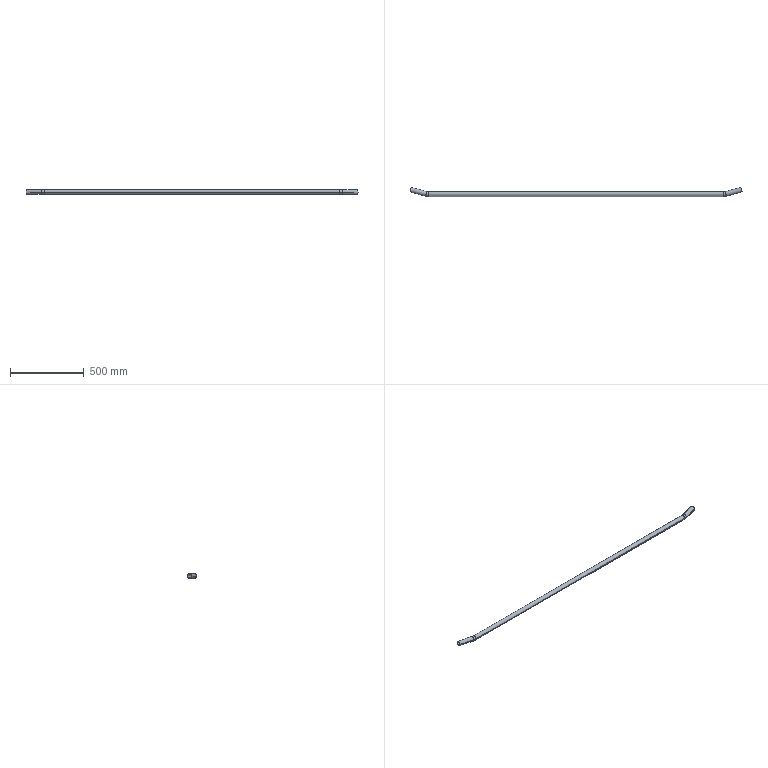Part | STEP file | DCV-000-033-2300L | 1 solid | 22 faces | box 2248 x 61.44 x 31.8 mm | volume 420872 mm3 | cylinder 12 | torus 8 | plane 2 | commonest cylinder face diameters 27.8 x6 31.8 x6
STEP:
#1=CARTESIAN_POINT('',(0.,0.,0.));
#2=DIRECTION('',(0.,0.,1.));
#3=DIRECTION('',(1.,0.,0.));
#4=AXIS2_PLACEMENT_3D('',#1,#2,#3);
#5=CARTESIAN_POINT('',(-1000.,13.9,0.));
#6=VERTEX_POINT('',#5);
#7=CARTESIAN_POINT('',(-1010.87,15.331,0.));
#8=VERTEX_POINT('',#7);
#9=CARTESIAN_POINT('',(-1000.,55.9,0.));
#10=DIRECTION('',(0.,0.,-1.));
#11=DIRECTION('',(-1.,0.,0.));
#12=AXIS2_PLACEMENT_3D('',#9,#10,#11);
#13=CIRCLE('',#12,42.);
#14=CARTESIAN_POINT('',(-1000.,55.9,0.));
#15=DIRECTION('',(0.,0.,-1.));
#16=DIRECTION('',(-1.,0.,0.));
#17=AXIS2_PLACEMENT_3D('',#14,#15,#16);
#18=TOROIDAL_SURFACE('',#17,55.9,13.9);
#19=CARTESIAN_POINT('',(0.,3.142));
#20=DIRECTION('',(1.,0.));
#21=VECTOR('',#20,1.);
#22=LINE('',#19,#21);
#23=(GEOMETRIC_REPRESENTATION_CONTEXT(2)PARAMETRIC_REPRESENTATION_CONTEXT()REPRESENTATION_CONTEXT('',''));
#24=DEFINITIONAL_REPRESENTATION('',(#22),#23);
#25=PCURVE('',#18,#24);
#26=CARTESIAN_POINT('',(-1000.,55.9,0.));
#27=DIRECTION('',(0.,0.,-1.));
#28=DIRECTION('',(-1.,0.,0.));
#29=AXIS2_PLACEMENT_3D('',#26,#27,#28);
#30=TOROIDAL_SURFACE('',#29,55.9,13.9);
#31=CARTESIAN_POINT('',(0.,3.142));
#32=DIRECTION('',(1.,0.));
#33=VECTOR('',#32,1.);
#34=LINE('',#31,#33);
#35=(GEOMETRIC_REPRESENTATION_CONTEXT(2)PARAMETRIC_REPRESENTATION_CONTEXT()REPRESENTATION_CONTEXT('',''));
#36=DEFINITIONAL_REPRESENTATION('',(#34),#35);
#37=PCURVE('',#30,#36);
#38=SURFACE_CURVE('',#13,(#25,#37),.PCURVE_S1.);
#39=EDGE_CURVE('',#6,#8,#38,.T.);
#40=ORIENTED_EDGE('',*,*,#39,.T.);
#41=CARTESIAN_POINT('',(-1018.066,-11.522,0.));
#42=VERTEX_POINT('',#41);
#43=CARTESIAN_POINT('',(-1014.468,1.905,0.));
#44=DIRECTION('',(-0.9659,0.2588,0.));
#45=DIRECTION('',(-0.2588,-0.9659,0.));
#46=AXIS2_PLACEMENT_3D('',#43,#44,#45);
#47=CIRCLE('',#46,13.9);
#48=CARTESIAN_POINT('',(4.974,6.283));
#49=DIRECTION('',(0.,-1.));
#50=VECTOR('',#49,1.);
#51=LINE('',#48,#50);
#52=(GEOMETRIC_REPRESENTATION_CONTEXT(2)PARAMETRIC_REPRESENTATION_CONTEXT()REPRESENTATION_CONTEXT('',''));
#53=DEFINITIONAL_REPRESENTATION('',(#51),#52);
#54=PCURVE('',#18,#53);
#55=CARTESIAN_POINT('',(-1014.468,1.905,0.));
#56=DIRECTION('',(-0.9659,0.2588,0.));
#57=DIRECTION('',(-0.2588,-0.9659,0.));
#58=AXIS2_PLACEMENT_3D('',#55,#56,#57);
#59=CYLINDRICAL_SURFACE('',#58,13.9);
#60=CARTESIAN_POINT('',(0.,0.));
#61=DIRECTION('',(1.,0.));
#62=VECTOR('',#61,1.);
#63=LINE('',#60,#62);
#64=(GEOMETRIC_REPRESENTATION_CONTEXT(2)PARAMETRIC_REPRESENTATION_CONTEXT()REPRESENTATION_CONTEXT('',''));
#65=DEFINITIONAL_REPRESENTATION('',(#63),#64);
#66=PCURVE('',#59,#65);
#67=SURFACE_CURVE('',#47,(#54,#66),.PCURVE_S1.);
#68=EDGE_CURVE('',#42,#8,#67,.T.);
#69=ORIENTED_EDGE('',*,*,#68,.F.);
#70=CARTESIAN_POINT('',(-1000.,-13.9,0.));
#71=VERTEX_POINT('',#70);
#72=CARTESIAN_POINT('',(-1000.,55.9,0.));
#73=DIRECTION('',(0.,0.,-1.));
#74=DIRECTION('',(-1.,0.,0.));
#75=AXIS2_PLACEMENT_3D('',#72,#73,#74);
#76=CIRCLE('',#75,69.8);
#77=CARTESIAN_POINT('',(0.,6.283));
#78=DIRECTION('',(1.,0.));
#79=VECTOR('',#78,1.);
#80=LINE('',#77,#79);
#81=(GEOMETRIC_REPRESENTATION_CONTEXT(2)PARAMETRIC_REPRESENTATION_CONTEXT()REPRESENTATION_CONTEXT('',''));
#82=DEFINITIONAL_REPRESENTATION('',(#80),#81);
#83=PCURVE('',#18,#82);
#84=CARTESIAN_POINT('',(0.,0.));
#85=DIRECTION('',(1.,0.));
#86=VECTOR('',#85,1.);
#87=LINE('',#84,#86);
#88=(GEOMETRIC_REPRESENTATION_CONTEXT(2)PARAMETRIC_REPRESENTATION_CONTEXT()REPRESENTATION_CONTEXT('',''));
#89=DEFINITIONAL_REPRESENTATION('',(#87),#88);
#90=PCURVE('',#30,#89);
#91=SURFACE_CURVE('',#76,(#83,#90),.PCURVE_S1.);
#92=EDGE_CURVE('',#71,#42,#91,.T.);
#93=ORIENTED_EDGE('',*,*,#92,.F.);
#94=CARTESIAN_POINT('',(-1000.,0.,0.));
#95=DIRECTION('',(-1.,0.,0.));
#96=DIRECTION('',(0.,-1.,0.));
#97=AXIS2_PLACEMENT_3D('',#94,#95,#96);
#98=CIRCLE('',#97,13.9);
#99=CARTESIAN_POINT('',(4.712,6.283));
#100=DIRECTION('',(0.,-1.));
#101=VECTOR('',#100,1.);
#102=LINE('',#99,#101);
#103=(GEOMETRIC_REPRESENTATION_CONTEXT(2)PARAMETRIC_REPRESENTATION_CONTEXT()REPRESENTATION_CONTEXT('',''));
#104=DEFINITIONAL_REPRESENTATION('',(#102),#103);
#105=PCURVE('',#18,#104);
#106=CARTESIAN_POINT('',(1000.,0.,0.));
#107=DIRECTION('',(-1.,0.,0.));
#108=DIRECTION('',(0.,-1.,0.));
#109=AXIS2_PLACEMENT_3D('',#106,#107,#108);
#110=CYLINDRICAL_SURFACE('',#109,13.9);
#111=CARTESIAN_POINT('',(0.,2000.));
#112=DIRECTION('',(1.,0.));
#113=VECTOR('',#112,1.);
#114=LINE('',#111,#113);
#115=(GEOMETRIC_REPRESENTATION_CONTEXT(2)PARAMETRIC_REPRESENTATION_CONTEXT()REPRESENTATION_CONTEXT('',''));
#116=DEFINITIONAL_REPRESENTATION('',(#114),#115);
#117=PCURVE('',#110,#116);
#118=SURFACE_CURVE('',#98,(#105,#117),.PCURVE_S1.);
#119=EDGE_CURVE('',#71,#6,#118,.T.);
#120=ORIENTED_EDGE('',*,*,#119,.T.);
#121=EDGE_LOOP('',(#40,#69,#93,#120));
#122=FACE_BOUND('',#121,.F.);
#123=ADVANCED_FACE('',(#122),#18,.F.);
#124=CARTESIAN_POINT('',(1010.87,15.331,0.));
#125=VERTEX_POINT('',#124);
#126=CARTESIAN_POINT('',(1000.,13.9,0.));
#127=VERTEX_POINT('',#126);
#128=CARTESIAN_POINT('',(1000.,55.9,0.));
#129=DIRECTION('',(0.,0.,-1.));
#130=DIRECTION('',(-1.,0.,0.));
#131=AXIS2_PLACEMENT_3D('',#128,#129,#130);
#132=CIRCLE('',#131,42.);
#133=CARTESIAN_POINT('',(1000.,55.9,0.));
#134=DIRECTION('',(0.,0.,-1.));
#135=DIRECTION('',(-1.,0.,0.));
#136=AXIS2_PLACEMENT_3D('',#133,#134,#135);
#137=TOROIDAL_SURFACE('',#136,55.9,13.9);
#138=CARTESIAN_POINT('',(0.,3.142));
#139=DIRECTION('',(1.,0.));
#140=VECTOR('',#139,1.);
#141=LINE('',#138,#140);
#142=(GEOMETRIC_REPRESENTATION_CONTEXT(2)PARAMETRIC_REPRESENTATION_CONTEXT()REPRESENTATION_CONTEXT('',''));
#143=DEFINITIONAL_REPRESENTATION('',(#141),#142);
#144=PCURVE('',#137,#143);
#145=CARTESIAN_POINT('',(1000.,55.9,0.));
#146=DIRECTION('',(0.,0.,-1.));
#147=DIRECTION('',(-1.,0.,0.));
#148=AXIS2_PLACEMENT_3D('',#145,#146,#147);
#149=TOROIDAL_SURFACE('',#148,55.9,13.9);
#150=CARTESIAN_POINT('',(0.,3.142));
#151=DIRECTION('',(1.,0.));
#152=VECTOR('',#151,1.);
#153=LINE('',#150,#152);
#154=(GEOMETRIC_REPRESENTATION_CONTEXT(2)PARAMETRIC_REPRESENTATION_CONTEXT()REPRESENTATION_CONTEXT('',''));
#155=DEFINITIONAL_REPRESENTATION('',(#153),#154);
#156=PCURVE('',#149,#155);
#157=SURFACE_CURVE('',#132,(#144,#156),.PCURVE_S1.);
#158=EDGE_CURVE('',#125,#127,#157,.T.);
#159=ORIENTED_EDGE('',*,*,#158,.T.);
#160=CARTESIAN_POINT('',(1000.,-13.9,0.));
#161=VERTEX_POINT('',#160);
#162=CARTESIAN_POINT('',(1000.,0.,0.));
#163=DIRECTION('',(-1.,0.,0.));
#164=DIRECTION('',(0.,-1.,0.));
#165=AXIS2_PLACEMENT_3D('',#162,#163,#164);
#166=CIRCLE('',#165,13.9);
#167=CARTESIAN_POINT('',(4.712,6.283));
#168=DIRECTION('',(0.,-1.));
#169=VECTOR('',#168,1.);
#170=LINE('',#167,#169);
#171=(GEOMETRIC_REPRESENTATION_CONTEXT(2)PARAMETRIC_REPRESENTATION_CONTEXT()REPRESENTATION_CONTEXT('',''));
#172=DEFINITIONAL_REPRESENTATION('',(#170),#171);
#173=PCURVE('',#137,#172);
#174=CARTESIAN_POINT('',(0.,0.));
#175=DIRECTION('',(1.,0.));
#176=VECTOR('',#175,1.);
#177=LINE('',#174,#176);
#178=(GEOMETRIC_REPRESENTATION_CONTEXT(2)PARAMETRIC_REPRESENTATION_CONTEXT()REPRESENTATION_CONTEXT('',''));
#179=DEFINITIONAL_REPRESENTATION('',(#177),#178);
#180=PCURVE('',#110,#179);
#181=SURFACE_CURVE('',#166,(#173,#180),.PCURVE_S1.);
#182=EDGE_CURVE('',#161,#127,#181,.T.);
#183=ORIENTED_EDGE('',*,*,#182,.F.);
#184=CARTESIAN_POINT('',(1018.066,-11.522,0.));
#185=VERTEX_POINT('',#184);
#186=CARTESIAN_POINT('',(1000.,55.9,0.));
#187=DIRECTION('',(0.,0.,-1.));
#188=DIRECTION('',(-1.,0.,0.));
#189=AXIS2_PLACEMENT_3D('',#186,#187,#188);
#190=CIRCLE('',#189,69.8);
#191=CARTESIAN_POINT('',(0.,6.283));
#192=DIRECTION('',(1.,0.));
#193=VECTOR('',#192,1.);
#194=LINE('',#191,#193);
#195=(GEOMETRIC_REPRESENTATION_CONTEXT(2)PARAMETRIC_REPRESENTATION_CONTEXT()REPRESENTATION_CONTEXT('',''));
#196=DEFINITIONAL_REPRESENTATION('',(#194),#195);
#197=PCURVE('',#137,#196);
#198=CARTESIAN_POINT('',(0.,0.));
#199=DIRECTION('',(1.,0.));
#200=VECTOR('',#199,1.);
#201=LINE('',#198,#200);
#202=(GEOMETRIC_REPRESENTATION_CONTEXT(2)PARAMETRIC_REPRESENTATION_CONTEXT()REPRESENTATION_CONTEXT('',''));
#203=DEFINITIONAL_REPRESENTATION('',(#201),#202);
#204=PCURVE('',#149,#203);
#205=SURFACE_CURVE('',#190,(#197,#204),.PCURVE_S1.);
#206=EDGE_CURVE('',#185,#161,#205,.T.);
#207=ORIENTED_EDGE('',*,*,#206,.F.);
#208=CARTESIAN_POINT('',(1014.468,1.905,0.));
#209=DIRECTION('',(-0.9659,-0.2588,0.));
#210=DIRECTION('',(0.2588,-0.9659,0.));
#211=AXIS2_PLACEMENT_3D('',#208,#209,#210);
#212=CIRCLE('',#211,13.9);
#213=CARTESIAN_POINT('',(4.451,6.283));
#214=DIRECTION('',(0.,-1.));
#215=VECTOR('',#214,1.);
#216=LINE('',#213,#215);
#217=(GEOMETRIC_REPRESENTATION_CONTEXT(2)PARAMETRIC_REPRESENTATION_CONTEXT()REPRESENTATION_CONTEXT('',''));
#218=DEFINITIONAL_REPRESENTATION('',(#216),#217);
#219=PCURVE('',#137,#218);
#220=CARTESIAN_POINT('',(1120.,30.182,0.));
#221=DIRECTION('',(-0.9659,-0.2588,0.));
#222=DIRECTION('',(0.2588,-0.9659,0.));
#223=AXIS2_PLACEMENT_3D('',#220,#221,#222);
#224=CYLINDRICAL_SURFACE('',#223,13.9);
#225=CARTESIAN_POINT('',(0.,109.255));
#226=DIRECTION('',(1.,0.));
#227=VECTOR('',#226,1.);
#228=LINE('',#225,#227);
#229=(GEOMETRIC_REPRESENTATION_CONTEXT(2)PARAMETRIC_REPRESENTATION_CONTEXT()REPRESENTATION_CONTEXT('',''));
#230=DEFINITIONAL_REPRESENTATION('',(#228),#229);
#231=PCURVE('',#224,#230);
#232=SURFACE_CURVE('',#212,(#219,#231),.PCURVE_S1.);
#233=EDGE_CURVE('',#185,#125,#232,.T.);
#234=ORIENTED_EDGE('',*,*,#233,.T.);
#235=EDGE_LOOP('',(#159,#183,#207,#234));
#236=FACE_BOUND('',#235,.F.);
#237=ADVANCED_FACE('',(#236),#137,.F.);
#238=CARTESIAN_POINT('',(-1000.,15.9,0.));
#239=VERTEX_POINT('',#238);
#240=CARTESIAN_POINT('',(-1000.,-15.9,0.));
#241=VERTEX_POINT('',#240);
#242=CARTESIAN_POINT('',(-1000.,0.,0.));
#243=DIRECTION('',(-1.,0.,0.));
#244=DIRECTION('',(0.,1.,0.));
#245=AXIS2_PLACEMENT_3D('',#242,#243,#244);
#246=CIRCLE('',#245,15.9);
#247=CARTESIAN_POINT('',(-1000.,55.9,0.));
#248=DIRECTION('',(0.,0.,-1.));
#249=DIRECTION('',(-1.,0.,0.));
#250=AXIS2_PLACEMENT_3D('',#247,#248,#249);
#251=TOROIDAL_SURFACE('',#250,55.9,15.9);
#252=CARTESIAN_POINT('',(4.712,3.142));
#253=DIRECTION('',(0.,-1.));
#254=VECTOR('',#253,1.);
#255=LINE('',#252,#254);
#256=(GEOMETRIC_REPRESENTATION_CONTEXT(2)PARAMETRIC_REPRESENTATION_CONTEXT()REPRESENTATION_CONTEXT('',''));
#257=DEFINITIONAL_REPRESENTATION('',(#255),#256);
#258=PCURVE('',#251,#257);
#259=CARTESIAN_POINT('',(1000.,0.,0.));
#260=DIRECTION('',(-1.,0.,0.));
#261=DIRECTION('',(0.,1.,0.));
#262=AXIS2_PLACEMENT_3D('',#259,#260,#261);
#263=CYLINDRICAL_SURFACE('',#262,15.9);
#264=CARTESIAN_POINT('',(0.,2000.));
#265=DIRECTION('',(1.,0.));
#266=VECTOR('',#265,1.);
#267=LINE('',#264,#266);
#268=(GEOMETRIC_REPRESENTATION_CONTEXT(2)PARAMETRIC_REPRESENTATION_CONTEXT()REPRESENTATION_CONTEXT('',''));
#269=DEFINITIONAL_REPRESENTATION('',(#267),#268);
#270=PCURVE('',#263,#269);
#271=SURFACE_CURVE('',#246,(#258,#270),.PCURVE_S1.);
#272=EDGE_CURVE('',#239,#241,#271,.T.);
#273=ORIENTED_EDGE('',*,*,#272,.T.);
#274=CARTESIAN_POINT('',(-1018.583,-13.453,0.));
#275=VERTEX_POINT('',#274);
#276=CARTESIAN_POINT('',(-1000.,55.9,0.));
#277=DIRECTION('',(0.,0.,-1.));
#278=DIRECTION('',(-1.,0.,0.));
#279=AXIS2_PLACEMENT_3D('',#276,#277,#278);
#280=CIRCLE('',#279,71.8);
#281=CARTESIAN_POINT('',(0.,0.));
#282=DIRECTION('',(1.,0.));
#283=VECTOR('',#282,1.);
#284=LINE('',#281,#283);
#285=(GEOMETRIC_REPRESENTATION_CONTEXT(2)PARAMETRIC_REPRESENTATION_CONTEXT()REPRESENTATION_CONTEXT('',''));
#286=DEFINITIONAL_REPRESENTATION('',(#284),#285);
#287=PCURVE('',#251,#286);
#288=CARTESIAN_POINT('',(-1000.,55.9,0.));
#289=DIRECTION('',(0.,0.,-1.));
#290=DIRECTION('',(-1.,0.,0.));
#291=AXIS2_PLACEMENT_3D('',#288,#289,#290);
#292=TOROIDAL_SURFACE('',#291,55.9,15.9);
#293=CARTESIAN_POINT('',(0.,6.283));
#294=DIRECTION('',(1.,0.));
#295=VECTOR('',#294,1.);
#296=LINE('',#293,#295);
#297=(GEOMETRIC_REPRESENTATION_CONTEXT(2)PARAMETRIC_REPRESENTATION_CONTEXT()REPRESENTATION_CONTEXT('',''));
#298=DEFINITIONAL_REPRESENTATION('',(#296),#297);
#299=PCURVE('',#292,#298);
#300=SURFACE_CURVE('',#280,(#287,#299),.PCURVE_S1.);
#301=EDGE_CURVE('',#241,#275,#300,.T.);
#302=ORIENTED_EDGE('',*,*,#301,.T.);
#303=CARTESIAN_POINT('',(-1010.353,17.263,0.));
#304=VERTEX_POINT('',#303);
#305=CARTESIAN_POINT('',(-1014.468,1.905,0.));
#306=DIRECTION('',(-0.9659,0.2588,0.));
#307=DIRECTION('',(0.2588,0.9659,0.));
#308=AXIS2_PLACEMENT_3D('',#305,#306,#307);
#309=CIRCLE('',#308,15.9);
#310=CARTESIAN_POINT('',(4.974,3.142));
#311=DIRECTION('',(0.,-1.));
#312=VECTOR('',#311,1.);
#313=LINE('',#310,#312);
#314=(GEOMETRIC_REPRESENTATION_CONTEXT(2)PARAMETRIC_REPRESENTATION_CONTEXT()REPRESENTATION_CONTEXT('',''));
#315=DEFINITIONAL_REPRESENTATION('',(#313),#314);
#316=PCURVE('',#251,#315);
#317=CARTESIAN_POINT('',(-1014.468,1.905,0.));
#318=DIRECTION('',(-0.9659,0.2588,0.));
#319=DIRECTION('',(0.2588,0.9659,0.));
#320=AXIS2_PLACEMENT_3D('',#317,#318,#319);
#321=CYLINDRICAL_SURFACE('',#320,15.9);
#322=CARTESIAN_POINT('',(0.,0.));
#323=DIRECTION('',(1.,0.));
#324=VECTOR('',#323,1.);
#325=LINE('',#322,#324);
#326=(GEOMETRIC_REPRESENTATION_CONTEXT(2)PARAMETRIC_REPRESENTATION_CONTEXT()REPRESENTATION_CONTEXT('',''));
#327=DEFINITIONAL_REPRESENTATION('',(#325),#326);
#328=PCURVE('',#321,#327);
#329=SURFACE_CURVE('',#309,(#316,#328),.PCURVE_S1.);
#330=EDGE_CURVE('',#304,#275,#329,.T.);
#331=ORIENTED_EDGE('',*,*,#330,.F.);
#332=CARTESIAN_POINT('',(-1000.,55.9,0.));
#333=DIRECTION('',(0.,0.,-1.));
#334=DIRECTION('',(-1.,0.,0.));
#335=AXIS2_PLACEMENT_3D('',#332,#333,#334);
#336=CIRCLE('',#335,40.);
#337=CARTESIAN_POINT('',(0.,3.142));
#338=DIRECTION('',(1.,0.));
#339=VECTOR('',#338,1.);
#340=LINE('',#337,#339);
#341=(GEOMETRIC_REPRESENTATION_CONTEXT(2)PARAMETRIC_REPRESENTATION_CONTEXT()REPRESENTATION_CONTEXT('',''));
#342=DEFINITIONAL_REPRESENTATION('',(#340),#341);
#343=PCURVE('',#251,#342);
#344=CARTESIAN_POINT('',(0.,3.142));
#345=DIRECTION('',(1.,0.));
#346=VECTOR('',#345,1.);
#347=LINE('',#344,#346);
#348=(GEOMETRIC_REPRESENTATION_CONTEXT(2)PARAMETRIC_REPRESENTATION_CONTEXT()REPRESENTATION_CONTEXT('',''));
#349=DEFINITIONAL_REPRESENTATION('',(#347),#348);
#350=PCURVE('',#292,#349);
#351=SURFACE_CURVE('',#336,(#343,#350),.PCURVE_S1.);
#352=EDGE_CURVE('',#239,#304,#351,.T.);
#353=ORIENTED_EDGE('',*,*,#352,.F.);
#354=EDGE_LOOP('',(#273,#302,#331,#353));
#355=FACE_BOUND('',#354,.T.);
#356=ADVANCED_FACE('',(#355),#251,.T.);
#357=CARTESIAN_POINT('',(1010.353,17.263,0.));
#358=VERTEX_POINT('',#357);
#359=CARTESIAN_POINT('',(1018.583,-13.453,0.));
#360=VERTEX_POINT('',#359);
#361=CARTESIAN_POINT('',(1014.468,1.905,0.));
#362=DIRECTION('',(-0.9659,-0.2588,0.));
#363=DIRECTION('',(-0.2588,0.9659,0.));
#364=AXIS2_PLACEMENT_3D('',#361,#362,#363);
#365=CIRCLE('',#364,15.9);
#366=CARTESIAN_POINT('',(1000.,55.9,0.));
#367=DIRECTION('',(0.,0.,-1.));
#368=DIRECTION('',(-1.,0.,0.));
#369=AXIS2_PLACEMENT_3D('',#366,#367,#368);
#370=TOROIDAL_SURFACE('',#369,55.9,15.9);
#371=CARTESIAN_POINT('',(4.451,3.142));
#372=DIRECTION('',(0.,-1.));
#373=VECTOR('',#372,1.);
#374=LINE('',#371,#373);
#375=(GEOMETRIC_REPRESENTATION_CONTEXT(2)PARAMETRIC_REPRESENTATION_CONTEXT()REPRESENTATION_CONTEXT('',''));
#376=DEFINITIONAL_REPRESENTATION('',(#374),#375);
#377=PCURVE('',#370,#376);
#378=CARTESIAN_POINT('',(1120.,30.182,0.));
#379=DIRECTION('',(-0.9659,-0.2588,0.));
#380=DIRECTION('',(-0.2588,0.9659,0.));
#381=AXIS2_PLACEMENT_3D('',#378,#379,#380);
#382=CYLINDRICAL_SURFACE('',#381,15.9);
#383=CARTESIAN_POINT('',(0.,109.255));
#384=DIRECTION('',(1.,0.));
#385=VECTOR('',#384,1.);
#386=LINE('',#383,#385);
#387=(GEOMETRIC_REPRESENTATION_CONTEXT(2)PARAMETRIC_REPRESENTATION_CONTEXT()REPRESENTATION_CONTEXT('',''));
#388=DEFINITIONAL_REPRESENTATION('',(#386),#387);
#389=PCURVE('',#382,#388);
#390=SURFACE_CURVE('',#365,(#377,#389),.PCURVE_S1.);
#391=EDGE_CURVE('',#358,#360,#390,.T.);
#392=ORIENTED_EDGE('',*,*,#391,.T.);
#393=CARTESIAN_POINT('',(1000.,-15.9,0.));
#394=VERTEX_POINT('',#393);
#395=CARTESIAN_POINT('',(1000.,55.9,0.));
#396=DIRECTION('',(0.,0.,-1.));
#397=DIRECTION('',(-1.,0.,0.));
#398=AXIS2_PLACEMENT_3D('',#395,#396,#397);
#399=CIRCLE('',#398,71.8);
#400=CARTESIAN_POINT('',(0.,0.));
#401=DIRECTION('',(1.,0.));
#402=VECTOR('',#401,1.);
#403=LINE('',#400,#402);
#404=(GEOMETRIC_REPRESENTATION_CONTEXT(2)PARAMETRIC_REPRESENTATION_CONTEXT()REPRESENTATION_CONTEXT('',''));
#405=DEFINITIONAL_REPRESENTATION('',(#403),#404);
#406=PCURVE('',#370,#405);
#407=CARTESIAN_POINT('',(1000.,55.9,0.));
#408=DIRECTION('',(0.,0.,-1.));
#409=DIRECTION('',(-1.,0.,0.));
#410=AXIS2_PLACEMENT_3D('',#407,#408,#409);
#411=TOROIDAL_SURFACE('',#410,55.9,15.9);
#412=CARTESIAN_POINT('',(0.,6.283));
#413=DIRECTION('',(1.,0.));
#414=VECTOR('',#413,1.);
#415=LINE('',#412,#414);
#416=(GEOMETRIC_REPRESENTATION_CONTEXT(2)PARAMETRIC_REPRESENTATION_CONTEXT()REPRESENTATION_CONTEXT('',''));
#417=DEFINITIONAL_REPRESENTATION('',(#415),#416);
#418=PCURVE('',#411,#417);
#419=SURFACE_CURVE('',#399,(#406,#418),.PCURVE_S1.);
#420=EDGE_CURVE('',#360,#394,#419,.T.);
#421=ORIENTED_EDGE('',*,*,#420,.T.);
#422=CARTESIAN_POINT('',(1000.,15.9,0.));
#423=VERTEX_POINT('',#422);
#424=CARTESIAN_POINT('',(1000.,0.,0.));
#425=DIRECTION('',(-1.,0.,0.));
#426=DIRECTION('',(0.,1.,0.));
#427=AXIS2_PLACEMENT_3D('',#424,#425,#426);
#428=CIRCLE('',#427,15.9);
#429=CARTESIAN_POINT('',(4.712,3.142));
#430=DIRECTION('',(0.,-1.));
#431=VECTOR('',#430,1.);
#432=LINE('',#429,#431);
#433=(GEOMETRIC_REPRESENTATION_CONTEXT(2)PARAMETRIC_REPRESENTATION_CONTEXT()REPRESENTATION_CONTEXT('',''));
#434=DEFINITIONAL_REPRESENTATION('',(#432),#433);
#435=PCURVE('',#370,#434);
#436=CARTESIAN_POINT('',(0.,0.));
#437=DIRECTION('',(1.,0.));
#438=VECTOR('',#437,1.);
#439=LINE('',#436,#438);
#440=(GEOMETRIC_REPRESENTATION_CONTEXT(2)PARAMETRIC_REPRESENTATION_CONTEXT()REPRESENTATION_CONTEXT('',''));
#441=DEFINITIONAL_REPRESENTATION('',(#439),#440);
#442=PCURVE('',#263,#441);
#443=SURFACE_CURVE('',#428,(#435,#442),.PCURVE_S1.);
#444=EDGE_CURVE('',#423,#394,#443,.T.);
#445=ORIENTED_EDGE('',*,*,#444,.F.);
#446=CARTESIAN_POINT('',(1000.,55.9,0.));
#447=DIRECTION('',(0.,0.,-1.));
#448=DIRECTION('',(-1.,0.,0.));
#449=AXIS2_PLACEMENT_3D('',#446,#447,#448);
#450=CIRCLE('',#449,40.);
#451=CARTESIAN_POINT('',(0.,3.142));
#452=DIRECTION('',(1.,0.));
#453=VECTOR('',#452,1.);
#454=LINE('',#451,#453);
#455=(GEOMETRIC_REPRESENTATION_CONTEXT(2)PARAMETRIC_REPRESENTATION_CONTEXT()REPRESENTATION_CONTEXT('',''));
#456=DEFINITIONAL_REPRESENTATION('',(#454),#455);
#457=PCURVE('',#370,#456);
#458=CARTESIAN_POINT('',(0.,3.142));
#459=DIRECTION('',(1.,0.));
#460=VECTOR('',#459,1.);
#461=LINE('',#458,#460);
#462=(GEOMETRIC_REPRESENTATION_CONTEXT(2)PARAMETRIC_REPRESENTATION_CONTEXT()REPRESENTATION_CONTEXT('',''));
#463=DEFINITIONAL_REPRESENTATION('',(#461),#462);
#464=PCURVE('',#411,#463);
#465=SURFACE_CURVE('',#450,(#457,#464),.PCURVE_S1.);
#466=EDGE_CURVE('',#358,#423,#465,.T.);
#467=ORIENTED_EDGE('',*,*,#466,.F.);
#468=EDGE_LOOP('',(#392,#421,#445,#467));
#469=FACE_BOUND('',#468,.T.);
#470=ADVANCED_FACE('',(#469),#370,.T.);
#471=CARTESIAN_POINT('',(-1123.598,16.756,0.));
#472=VERTEX_POINT('',#471);
#473=CARTESIAN_POINT('',(-1018.066,-11.522,0.));
#474=DIRECTION('',(-0.9659,0.2588,0.));
#475=VECTOR('',#474,1.);
#476=LINE('',#473,#475);
#477=CARTESIAN_POINT('',(-1014.468,1.905,0.));
#478=DIRECTION('',(-0.9659,0.2588,0.));
#479=DIRECTION('',(-0.2588,-0.9659,0.));
#480=AXIS2_PLACEMENT_3D('',#477,#478,#479);
#481=CYLINDRICAL_SURFACE('',#480,13.9);
#482=CARTESIAN_POINT('',(6.283,0.));
#483=DIRECTION('',(0.,1.));
#484=VECTOR('',#483,1.);
#485=LINE('',#482,#484);
#486=(GEOMETRIC_REPRESENTATION_CONTEXT(2)PARAMETRIC_REPRESENTATION_CONTEXT()REPRESENTATION_CONTEXT('',''));
#487=DEFINITIONAL_REPRESENTATION('',(#485),#486);
#488=PCURVE('',#481,#487);
#489=CARTESIAN_POINT('',(0.,0.));
#490=DIRECTION('',(0.,1.));
#491=VECTOR('',#490,1.);
#492=LINE('',#489,#491);
#493=(GEOMETRIC_REPRESENTATION_CONTEXT(2)PARAMETRIC_REPRESENTATION_CONTEXT()REPRESENTATION_CONTEXT('',''));
#494=DEFINITIONAL_REPRESENTATION('',(#492),#493);
#495=PCURVE('',#59,#494);
#496=SURFACE_CURVE('',#476,(#488,#495),.PCURVE_S1.);
#497=EDGE_CURVE('',#42,#472,#496,.T.);
#498=ORIENTED_EDGE('',*,*,#497,.T.);
#499=CARTESIAN_POINT('',(-1116.402,43.608,0.));
#500=VERTEX_POINT('',#499);
#501=CARTESIAN_POINT('',(-1120.,30.182,0.));
#502=DIRECTION('',(0.9659,-0.2588,0.));
#503=DIRECTION('',(-0.2588,-0.9659,0.));
#504=AXIS2_PLACEMENT_3D('',#501,#502,#503);
#505=CIRCLE('',#504,13.9);
#506=CARTESIAN_POINT('',(6.283,109.255));
#507=DIRECTION('',(-1.,0.));
#508=VECTOR('',#507,1.);
#509=LINE('',#506,#508);
#510=(GEOMETRIC_REPRESENTATION_CONTEXT(2)PARAMETRIC_REPRESENTATION_CONTEXT()REPRESENTATION_CONTEXT('',''));
#511=DEFINITIONAL_REPRESENTATION('',(#509),#510);
#512=PCURVE('',#481,#511);
#513=CARTESIAN_POINT('',(-1120.,30.182,0.));
#514=DIRECTION('',(0.9659,-0.2588,0.));
#515=DIRECTION('',(0.,0.,-1.));
#516=AXIS2_PLACEMENT_3D('',#513,#514,#515);
#517=PLANE('',#516);
#518=CARTESIAN_POINT('',(0.,0.));
#519=DIRECTION('',(0.,-1.));
#520=AXIS2_PLACEMENT_2D('',#518,#519);
#521=CIRCLE('',#520,13.9);
#522=(GEOMETRIC_REPRESENTATION_CONTEXT(2)PARAMETRIC_REPRESENTATION_CONTEXT()REPRESENTATION_CONTEXT('',''));
#523=DEFINITIONAL_REPRESENTATION('',(#521),#522);
#524=PCURVE('',#517,#523);
#525=SURFACE_CURVE('',#505,(#512,#524),.PCURVE_S1.);
#526=EDGE_CURVE('',#472,#500,#525,.T.);
#527=ORIENTED_EDGE('',*,*,#526,.T.);
#528=CARTESIAN_POINT('',(-1010.87,15.331,0.));
#529=DIRECTION('',(-0.9659,0.2588,0.));
#530=VECTOR('',#529,1.);
#531=LINE('',#528,#530);
#532=CARTESIAN_POINT('',(3.142,0.));
#533=DIRECTION('',(0.,1.));
#534=VECTOR('',#533,1.);
#535=LINE('',#532,#534);
#536=(GEOMETRIC_REPRESENTATION_CONTEXT(2)PARAMETRIC_REPRESENTATION_CONTEXT()REPRESENTATION_CONTEXT('',''));
#537=DEFINITIONAL_REPRESENTATION('',(#535),#536);
#538=PCURVE('',#481,#537);
#539=CARTESIAN_POINT('',(3.142,0.));
#540=DIRECTION('',(0.,1.));
#541=VECTOR('',#540,1.);
#542=LINE('',#539,#541);
#543=(GEOMETRIC_REPRESENTATION_CONTEXT(2)PARAMETRIC_REPRESENTATION_CONTEXT()REPRESENTATION_CONTEXT('',''));
#544=DEFINITIONAL_REPRESENTATION('',(#542),#543);
#545=PCURVE('',#59,#544);
#546=SURFACE_CURVE('',#531,(#538,#545),.PCURVE_S1.);
#547=EDGE_CURVE('',#8,#500,#546,.T.);
#548=ORIENTED_EDGE('',*,*,#547,.F.);
#549=CARTESIAN_POINT('',(-1014.468,1.905,0.));
#550=DIRECTION('',(-0.9659,0.2588,0.));
#551=DIRECTION('',(-0.2588,-0.9659,0.));
#552=AXIS2_PLACEMENT_3D('',#549,#550,#551);
#553=CIRCLE('',#552,13.9);
#554=CARTESIAN_POINT('',(0.,0.));
#555=DIRECTION('',(1.,0.));
#556=VECTOR('',#555,1.);
#557=LINE('',#554,#556);
#558=(GEOMETRIC_REPRESENTATION_CONTEXT(2)PARAMETRIC_REPRESENTATION_CONTEXT()REPRESENTATION_CONTEXT('',''));
#559=DEFINITIONAL_REPRESENTATION('',(#557),#558);
#560=PCURVE('',#481,#559);
#561=CARTESIAN_POINT('',(4.974,6.283));
#562=DIRECTION('',(0.,-1.));
#563=VECTOR('',#562,1.);
#564=LINE('',#561,#563);
#565=(GEOMETRIC_REPRESENTATION_CONTEXT(2)PARAMETRIC_REPRESENTATION_CONTEXT()REPRESENTATION_CONTEXT('',''));
#566=DEFINITIONAL_REPRESENTATION('',(#564),#565);
#567=PCURVE('',#30,#566);
#568=SURFACE_CURVE('',#553,(#560,#567),.PCURVE_S1.);
#569=EDGE_CURVE('',#8,#42,#568,.T.);
#570=ORIENTED_EDGE('',*,*,#569,.T.);
#571=EDGE_LOOP('',(#498,#527,#548,#570));
#572=FACE_BOUND('',#571,.F.);
#573=ADVANCED_FACE('',(#572),#481,.F.);
#574=CARTESIAN_POINT('',(1000.,-13.9,0.));
#575=DIRECTION('',(-1.,0.,0.));
#576=VECTOR('',#575,1.);
#577=LINE('',#574,#576);
#578=CARTESIAN_POINT('',(1000.,0.,0.));
#579=DIRECTION('',(-1.,0.,0.));
#580=DIRECTION('',(0.,-1.,0.));
#581=AXIS2_PLACEMENT_3D('',#578,#579,#580);
#582=CYLINDRICAL_SURFACE('',#581,13.9);
#583=CARTESIAN_POINT('',(6.283,0.));
#584=DIRECTION('',(0.,1.));
#585=VECTOR('',#584,1.);
#586=LINE('',#583,#585);
#587=(GEOMETRIC_REPRESENTATION_CONTEXT(2)PARAMETRIC_REPRESENTATION_CONTEXT()REPRESENTATION_CONTEXT('',''));
#588=DEFINITIONAL_REPRESENTATION('',(#586),#587);
#589=PCURVE('',#582,#588);
#590=CARTESIAN_POINT('',(0.,0.));
#591=DIRECTION('',(0.,1.));
#592=VECTOR('',#591,1.);
#593=LINE('',#590,#592);
#594=(GEOMETRIC_REPRESENTATION_CONTEXT(2)PARAMETRIC_REPRESENTATION_CONTEXT()REPRESENTATION_CONTEXT('',''));
#595=DEFINITIONAL_REPRESENTATION('',(#593),#594);
#596=PCURVE('',#110,#595);
#597=SURFACE_CURVE('',#577,(#589,#596),.PCURVE_S1.);
#598=EDGE_CURVE('',#161,#71,#597,.T.);
#599=ORIENTED_EDGE('',*,*,#598,.T.);
#600=CARTESIAN_POINT('',(-1000.,0.,0.));
#601=DIRECTION('',(-1.,0.,0.));
#602=DIRECTION('',(0.,-1.,0.));
#603=AXIS2_PLACEMENT_3D('',#600,#601,#602);
#604=CIRCLE('',#603,13.9);
#605=CARTESIAN_POINT('',(0.,2000.));
#606=DIRECTION('',(1.,0.));
#607=VECTOR('',#606,1.);
#608=LINE('',#605,#607);
#609=(GEOMETRIC_REPRESENTATION_CONTEXT(2)PARAMETRIC_REPRESENTATION_CONTEXT()REPRESENTATION_CONTEXT('',''));
#610=DEFINITIONAL_REPRESENTATION('',(#608),#609);
#611=PCURVE('',#582,#610);
#612=CARTESIAN_POINT('',(4.712,6.283));
#613=DIRECTION('',(0.,-1.));
#614=VECTOR('',#613,1.);
#615=LINE('',#612,#614);
#616=(GEOMETRIC_REPRESENTATION_CONTEXT(2)PARAMETRIC_REPRESENTATION_CONTEXT()REPRESENTATION_CONTEXT('',''));
#617=DEFINITIONAL_REPRESENTATION('',(#615),#616);
#618=PCURVE('',#30,#617);
#619=SURFACE_CURVE('',#604,(#611,#618),.PCURVE_S1.);
#620=EDGE_CURVE('',#6,#71,#619,.T.);
#621=ORIENTED_EDGE('',*,*,#620,.F.);
#622=CARTESIAN_POINT('',(1000.,13.9,0.));
#623=DIRECTION('',(-1.,0.,0.));
#624=VECTOR('',#623,1.);
#625=LINE('',#622,#624);
#626=CARTESIAN_POINT('',(3.142,0.));
#627=DIRECTION('',(0.,1.));
#628=VECTOR('',#627,1.);
#629=LINE('',#626,#628);
#630=(GEOMETRIC_REPRESENTATION_CONTEXT(2)PARAMETRIC_REPRESENTATION_CONTEXT()REPRESENTATION_CONTEXT('',''));
#631=DEFINITIONAL_REPRESENTATION('',(#629),#630);
#632=PCURVE('',#582,#631);
#633=CARTESIAN_POINT('',(3.142,0.));
#634=DIRECTION('',(0.,1.));
#635=VECTOR('',#634,1.);
#636=LINE('',#633,#635);
#637=(GEOMETRIC_REPRESENTATION_CONTEXT(2)PARAMETRIC_REPRESENTATION_CONTEXT()REPRESENTATION_CONTEXT('',''));
#638=DEFINITIONAL_REPRESENTATION('',(#636),#637);
#639=PCURVE('',#110,#638);
#640=SURFACE_CURVE('',#625,(#632,#639),.PCURVE_S1.);
#641=EDGE_CURVE('',#127,#6,#640,.T.);
#642=ORIENTED_EDGE('',*,*,#641,.F.);
#643=CARTESIAN_POINT('',(1000.,0.,0.));
#644=DIRECTION('',(-1.,0.,0.));
#645=DIRECTION('',(0.,-1.,0.));
#646=AXIS2_PLACEMENT_3D('',#643,#644,#645);
#647=CIRCLE('',#646,13.9);
#648=CARTESIAN_POINT('',(0.,0.));
#649=DIRECTION('',(1.,0.));
#650=VECTOR('',#649,1.);
#651=LINE('',#648,#650);
#652=(GEOMETRIC_REPRESENTATION_CONTEXT(2)PARAMETRIC_REPRESENTATION_CONTEXT()REPRESENTATION_CONTEXT('',''));
#653=DEFINITIONAL_REPRESENTATION('',(#651),#652);
#654=PCURVE('',#582,#653);
#655=CARTESIAN_POINT('',(4.712,6.283));
#656=DIRECTION('',(0.,-1.));
#657=VECTOR('',#656,1.);
#658=LINE('',#655,#657);
#659=(GEOMETRIC_REPRESENTATION_CONTEXT(2)PARAMETRIC_REPRESENTATION_CONTEXT()REPRESENTATION_CONTEXT('',''));
#660=DEFINITIONAL_REPRESENTATION('',(#658),#659);
#661=PCURVE('',#149,#660);
#662=SURFACE_CURVE('',#647,(#654,#661),.PCURVE_S1.);
#663=EDGE_CURVE('',#127,#161,#662,.T.);
#664=ORIENTED_EDGE('',*,*,#663,.T.);
#665=EDGE_LOOP('',(#599,#621,#642,#664));
#666=FACE_BOUND('',#665,.F.);
#667=ADVANCED_FACE('',(#666),#582,.F.);
#668=CARTESIAN_POINT('',(1123.598,16.756,0.));
#669=VERTEX_POINT('',#668);
#670=CARTESIAN_POINT('',(1123.598,16.756,0.));
#671=DIRECTION('',(-0.9659,-0.2588,0.));
#672=VECTOR('',#671,1.);
#673=LINE('',#670,#672);
#674=CARTESIAN_POINT('',(1120.,30.182,0.));
#675=DIRECTION('',(-0.9659,-0.2588,0.));
#676=DIRECTION('',(0.2588,-0.9659,0.));
#677=AXIS2_PLACEMENT_3D('',#674,#675,#676);
#678=CYLINDRICAL_SURFACE('',#677,13.9);
#679=CARTESIAN_POINT('',(6.283,0.));
#680=DIRECTION('',(0.,1.));
#681=VECTOR('',#680,1.);
#682=LINE('',#679,#681);
#683=(GEOMETRIC_REPRESENTATION_CONTEXT(2)PARAMETRIC_REPRESENTATION_CONTEXT()REPRESENTATION_CONTEXT('',''));
#684=DEFINITIONAL_REPRESENTATION('',(#682),#683);
#685=PCURVE('',#678,#684);
#686=CARTESIAN_POINT('',(0.,0.));
#687=DIRECTION('',(0.,1.));
#688=VECTOR('',#687,1.);
#689=LINE('',#686,#688);
#690=(GEOMETRIC_REPRESENTATION_CONTEXT(2)PARAMETRIC_REPRESENTATION_CONTEXT()REPRESENTATION_CONTEXT('',''));
#691=DEFINITIONAL_REPRESENTATION('',(#689),#690);
#692=PCURVE('',#224,#691);
#693=SURFACE_CURVE('',#673,(#685,#692),.PCURVE_S1.);
#694=EDGE_CURVE('',#669,#185,#693,.T.);
#695=ORIENTED_EDGE('',*,*,#694,.T.);
#696=CARTESIAN_POINT('',(1014.468,1.905,0.));
#697=DIRECTION('',(-0.9659,-0.2588,0.));
#698=DIRECTION('',(0.2588,-0.9659,0.));
#699=AXIS2_PLACEMENT_3D('',#696,#697,#698);
#700=CIRCLE('',#699,13.9);
#701=CARTESIAN_POINT('',(0.,109.255));
#702=DIRECTION('',(1.,0.));
#703=VECTOR('',#702,1.);
#704=LINE('',#701,#703);
#705=(GEOMETRIC_REPRESENTATION_CONTEXT(2)PARAMETRIC_REPRESENTATION_CONTEXT()REPRESENTATION_CONTEXT('',''));
#706=DEFINITIONAL_REPRESENTATION('',(#704),#705);
#707=PCURVE('',#678,#706);
#708=CARTESIAN_POINT('',(4.451,6.283));
#709=DIRECTION('',(0.,-1.));
#710=VECTOR('',#709,1.);
#711=LINE('',#708,#710);
#712=(GEOMETRIC_REPRESENTATION_CONTEXT(2)PARAMETRIC_REPRESENTATION_CONTEXT()REPRESENTATION_CONTEXT('',''));
#713=DEFINITIONAL_REPRESENTATION('',(#711),#712);
#714=PCURVE('',#149,#713);
#715=SURFACE_CURVE('',#700,(#707,#714),.PCURVE_S1.);
#716=EDGE_CURVE('',#125,#185,#715,.T.);
#717=ORIENTED_EDGE('',*,*,#716,.F.);
#718=CARTESIAN_POINT('',(1116.402,43.608,0.));
#719=VERTEX_POINT('',#718);
#720=CARTESIAN_POINT('',(1116.402,43.608,0.));
#721=DIRECTION('',(-0.9659,-0.2588,0.));
#722=VECTOR('',#721,1.);
#723=LINE('',#720,#722);
#724=CARTESIAN_POINT('',(3.142,0.));
#725=DIRECTION('',(0.,1.));
#726=VECTOR('',#725,1.);
#727=LINE('',#724,#726);
#728=(GEOMETRIC_REPRESENTATION_CONTEXT(2)PARAMETRIC_REPRESENTATION_CONTEXT()REPRESENTATION_CONTEXT('',''));
#729=DEFINITIONAL_REPRESENTATION('',(#727),#728);
#730=PCURVE('',#678,#729);
#731=CARTESIAN_POINT('',(3.142,0.));
#732=DIRECTION('',(0.,1.));
#733=VECTOR('',#732,1.);
#734=LINE('',#731,#733);
#735=(GEOMETRIC_REPRESENTATION_CONTEXT(2)PARAMETRIC_REPRESENTATION_CONTEXT()REPRESENTATION_CONTEXT('',''));
#736=DEFINITIONAL_REPRESENTATION('',(#734),#735);
#737=PCURVE('',#224,#736);
#738=SURFACE_CURVE('',#723,(#730,#737),.PCURVE_S1.);
#739=EDGE_CURVE('',#719,#125,#738,.T.);
#740=ORIENTED_EDGE('',*,*,#739,.F.);
#741=CARTESIAN_POINT('',(1120.,30.182,0.));
#742=DIRECTION('',(-0.9659,-0.2588,0.));
#743=DIRECTION('',(0.2588,-0.9659,0.));
#744=AXIS2_PLACEMENT_3D('',#741,#742,#743);
#745=CIRCLE('',#744,13.9);
#746=CARTESIAN_POINT('',(0.,0.));
#747=DIRECTION('',(1.,0.));
#748=VECTOR('',#747,1.);
#749=LINE('',#746,#748);
#750=(GEOMETRIC_REPRESENTATION_CONTEXT(2)PARAMETRIC_REPRESENTATION_CONTEXT()REPRESENTATION_CONTEXT('',''));
#751=DEFINITIONAL_REPRESENTATION('',(#749),#750);
#752=PCURVE('',#678,#751);
#753=CARTESIAN_POINT('',(1120.,30.182,0.));
#754=DIRECTION('',(0.9659,0.2588,0.));
#755=DIRECTION('',(0.,0.,-1.));
#756=AXIS2_PLACEMENT_3D('',#753,#754,#755);
#757=PLANE('',#756);
#758=CARTESIAN_POINT('',(0.,-13.9));
#759=CARTESIAN_POINT('',(-24.076,-13.9));
#760=CARTESIAN_POINT('',(-12.038,6.95));
#761=CARTESIAN_POINT('',(0.,27.8));
#762=CARTESIAN_POINT('',(12.038,6.95));
#763=CARTESIAN_POINT('',(24.076,-13.9));
#764=CARTESIAN_POINT('',(0.,-13.9));
#765=(BOUNDED_CURVE()B_SPLINE_CURVE(2,(#758,#759,#760,#761,#762,#763,#764),.UNSPECIFIED.,.T.,.F.)B_SPLINE_CURVE_WITH_KNOTS((1,2,2,2,2,1),(-2.094,0.,2.094,4.189,6.283,8.378),.UNSPECIFIED.)CURVE()GEOMETRIC_REPRESENTATION_ITEM()RATIONAL_B_SPLINE_CURVE((1.,0.5,1.,0.5,1.,0.5,1.))REPRESENTATION_ITEM(''));
#766=(GEOMETRIC_REPRESENTATION_CONTEXT(2)PARAMETRIC_REPRESENTATION_CONTEXT()REPRESENTATION_CONTEXT('',''));
#767=DEFINITIONAL_REPRESENTATION('',(#765),#766);
#768=PCURVE('',#757,#767);
#769=SURFACE_CURVE('',#745,(#752,#768),.PCURVE_S1.);
#770=EDGE_CURVE('',#719,#669,#769,.T.);
#771=ORIENTED_EDGE('',*,*,#770,.T.);
#772=EDGE_LOOP('',(#695,#717,#740,#771));
#773=FACE_BOUND('',#772,.F.);
#774=ADVANCED_FACE('',(#773),#678,.F.);
#775=ORIENTED_EDGE('',*,*,#330,.T.);
#776=CARTESIAN_POINT('',(-1124.115,14.824,0.));
#777=VERTEX_POINT('',#776);
#778=CARTESIAN_POINT('',(-1018.583,-13.453,0.));
#779=DIRECTION('',(-0.9659,0.2588,0.));
#780=VECTOR('',#779,1.);
#781=LINE('',#778,#780);
#782=CARTESIAN_POINT('',(3.142,0.));
#783=DIRECTION('',(0.,1.));
#784=VECTOR('',#783,1.);
#785=LINE('',#782,#784);
#786=(GEOMETRIC_REPRESENTATION_CONTEXT(2)PARAMETRIC_REPRESENTATION_CONTEXT()REPRESENTATION_CONTEXT('',''));
#787=DEFINITIONAL_REPRESENTATION('',(#785),#786);
#788=PCURVE('',#321,#787);
#789=CARTESIAN_POINT('',(-1014.468,1.905,0.));
#790=DIRECTION('',(-0.9659,0.2588,0.));
#791=DIRECTION('',(0.2588,0.9659,0.));
#792=AXIS2_PLACEMENT_3D('',#789,#790,#791);
#793=CYLINDRICAL_SURFACE('',#792,15.9);
#794=CARTESIAN_POINT('',(3.142,0.));
#795=DIRECTION('',(0.,1.));
#796=VECTOR('',#795,1.);
#797=LINE('',#794,#796);
#798=(GEOMETRIC_REPRESENTATION_CONTEXT(2)PARAMETRIC_REPRESENTATION_CONTEXT()REPRESENTATION_CONTEXT('',''));
#799=DEFINITIONAL_REPRESENTATION('',(#797),#798);
#800=PCURVE('',#793,#799);
#801=SURFACE_CURVE('',#781,(#788,#800),.PCURVE_S1.);
#802=EDGE_CURVE('',#275,#777,#801,.T.);
#803=ORIENTED_EDGE('',*,*,#802,.T.);
#804=CARTESIAN_POINT('',(-1115.885,45.54,0.));
#805=VERTEX_POINT('',#804);
#806=CARTESIAN_POINT('',(-1120.,30.182,0.));
#807=DIRECTION('',(-0.9659,0.2588,0.));
#808=DIRECTION('',(0.2588,0.9659,0.));
#809=AXIS2_PLACEMENT_3D('',#806,#807,#808);
#810=CIRCLE('',#809,15.9);
#811=CARTESIAN_POINT('',(0.,109.255));
#812=DIRECTION('',(1.,0.));
#813=VECTOR('',#812,1.);
#814=LINE('',#811,#813);
#815=(GEOMETRIC_REPRESENTATION_CONTEXT(2)PARAMETRIC_REPRESENTATION_CONTEXT()REPRESENTATION_CONTEXT('',''));
#816=DEFINITIONAL_REPRESENTATION('',(#814),#815);
#817=PCURVE('',#321,#816);
#818=CARTESIAN_POINT('',(0.,15.9));
#819=CARTESIAN_POINT('',(27.54,15.9));
#820=CARTESIAN_POINT('',(13.77,-7.95));
#821=CARTESIAN_POINT('',(0.,-31.8));
#822=CARTESIAN_POINT('',(-13.77,-7.95));
#823=CARTESIAN_POINT('',(-27.54,15.9));
#824=CARTESIAN_POINT('',(0.,15.9));
#825=(BOUNDED_CURVE()B_SPLINE_CURVE(2,(#818,#819,#820,#821,#822,#823,#824),.UNSPECIFIED.,.T.,.F.)B_SPLINE_CURVE_WITH_KNOTS((1,2,2,2,2,1),(-2.094,0.,2.094,4.189,6.283,8.378),.UNSPECIFIED.)CURVE()GEOMETRIC_REPRESENTATION_ITEM()RATIONAL_B_SPLINE_CURVE((1.,0.5,1.,0.5,1.,0.5,1.))REPRESENTATION_ITEM(''));
#826=(GEOMETRIC_REPRESENTATION_CONTEXT(2)PARAMETRIC_REPRESENTATION_CONTEXT()REPRESENTATION_CONTEXT('',''));
#827=DEFINITIONAL_REPRESENTATION('',(#825),#826);
#828=PCURVE('',#517,#827);
#829=SURFACE_CURVE('',#810,(#817,#828),.PCURVE_S1.);
#830=EDGE_CURVE('',#805,#777,#829,.T.);
#831=ORIENTED_EDGE('',*,*,#830,.F.);
#832=CARTESIAN_POINT('',(-1010.353,17.263,0.));
#833=DIRECTION('',(-0.9659,0.2588,0.));
#834=VECTOR('',#833,1.);
#835=LINE('',#832,#834);
#836=CARTESIAN_POINT('',(0.,0.));
#837=DIRECTION('',(0.,1.));
#838=VECTOR('',#837,1.);
#839=LINE('',#836,#838);
#840=(GEOMETRIC_REPRESENTATION_CONTEXT(2)PARAMETRIC_REPRESENTATION_CONTEXT()REPRESENTATION_CONTEXT('',''));
#841=DEFINITIONAL_REPRESENTATION('',(#839),#840);
#842=PCURVE('',#321,#841);
#843=CARTESIAN_POINT('',(6.283,0.));
#844=DIRECTION('',(0.,1.));
#845=VECTOR('',#844,1.);
#846=LINE('',#843,#845);
#847=(GEOMETRIC_REPRESENTATION_CONTEXT(2)PARAMETRIC_REPRESENTATION_CONTEXT()REPRESENTATION_CONTEXT('',''));
#848=DEFINITIONAL_REPRESENTATION('',(#846),#847);
#849=PCURVE('',#793,#848);
#850=SURFACE_CURVE('',#835,(#842,#849),.PCURVE_S1.);
#851=EDGE_CURVE('',#304,#805,#850,.T.);
#852=ORIENTED_EDGE('',*,*,#851,.F.);
#853=EDGE_LOOP('',(#775,#803,#831,#852));
#854=FACE_BOUND('',#853,.T.);
#855=ADVANCED_FACE('',(#854),#321,.T.);
#856=ORIENTED_EDGE('',*,*,#444,.T.);
#857=CARTESIAN_POINT('',(1000.,-15.9,0.));
#858=DIRECTION('',(-1.,0.,0.));
#859=VECTOR('',#858,1.);
#860=LINE('',#857,#859);
#861=CARTESIAN_POINT('',(3.142,0.));
#862=DIRECTION('',(0.,1.));
#863=VECTOR('',#862,1.);
#864=LINE('',#861,#863);
#865=(GEOMETRIC_REPRESENTATION_CONTEXT(2)PARAMETRIC_REPRESENTATION_CONTEXT()REPRESENTATION_CONTEXT('',''));
#866=DEFINITIONAL_REPRESENTATION('',(#864),#865);
#867=PCURVE('',#263,#866);
#868=CARTESIAN_POINT('',(1000.,0.,0.));
#869=DIRECTION('',(-1.,0.,0.));
#870=DIRECTION('',(0.,1.,0.));
#871=AXIS2_PLACEMENT_3D('',#868,#869,#870);
#872=CYLINDRICAL_SURFACE('',#871,15.9);
#873=CARTESIAN_POINT('',(3.142,0.));
#874=DIRECTION('',(0.,1.));
#875=VECTOR('',#874,1.);
#876=LINE('',#873,#875);
#877=(GEOMETRIC_REPRESENTATION_CONTEXT(2)PARAMETRIC_REPRESENTATION_CONTEXT()REPRESENTATION_CONTEXT('',''));
#878=DEFINITIONAL_REPRESENTATION('',(#876),#877);
#879=PCURVE('',#872,#878);
#880=SURFACE_CURVE('',#860,(#867,#879),.PCURVE_S1.);
#881=EDGE_CURVE('',#394,#241,#880,.T.);
#882=ORIENTED_EDGE('',*,*,#881,.T.);
#883=ORIENTED_EDGE('',*,*,#272,.F.);
#884=CARTESIAN_POINT('',(1000.,15.9,0.));
#885=DIRECTION('',(-1.,0.,0.));
#886=VECTOR('',#885,1.);
#887=LINE('',#884,#886);
#888=CARTESIAN_POINT('',(0.,0.));
#889=DIRECTION('',(0.,1.));
#890=VECTOR('',#889,1.);
#891=LINE('',#888,#890);
#892=(GEOMETRIC_REPRESENTATION_CONTEXT(2)PARAMETRIC_REPRESENTATION_CONTEXT()REPRESENTATION_CONTEXT('',''));
#893=DEFINITIONAL_REPRESENTATION('',(#891),#892);
#894=PCURVE('',#263,#893);
#895=CARTESIAN_POINT('',(6.283,0.));
#896=DIRECTION('',(0.,1.));
#897=VECTOR('',#896,1.);
#898=LINE('',#895,#897);
#899=(GEOMETRIC_REPRESENTATION_CONTEXT(2)PARAMETRIC_REPRESENTATION_CONTEXT()REPRESENTATION_CONTEXT('',''));
#900=DEFINITIONAL_REPRESENTATION('',(#898),#899);
#901=PCURVE('',#872,#900);
#902=SURFACE_CURVE('',#887,(#894,#901),.PCURVE_S1.);
#903=EDGE_CURVE('',#423,#239,#902,.T.);
#904=ORIENTED_EDGE('',*,*,#903,.F.);
#905=EDGE_LOOP('',(#856,#882,#883,#904));
#906=FACE_BOUND('',#905,.T.);
#907=ADVANCED_FACE('',(#906),#263,.T.);
#908=CARTESIAN_POINT('',(1124.115,14.824,0.));
#909=VERTEX_POINT('',#908);
#910=CARTESIAN_POINT('',(1115.885,45.54,0.));
#911=VERTEX_POINT('',#910);
#912=CARTESIAN_POINT('',(1120.,30.182,0.));
#913=DIRECTION('',(0.9659,0.2588,0.));
#914=DIRECTION('',(-0.2588,0.9659,0.));
#915=AXIS2_PLACEMENT_3D('',#912,#913,#914);
#916=CIRCLE('',#915,15.9);
#917=CARTESIAN_POINT('',(6.283,0.));
#918=DIRECTION('',(-1.,0.));
#919=VECTOR('',#918,1.);
#920=LINE('',#917,#919);
#921=(GEOMETRIC_REPRESENTATION_CONTEXT(2)PARAMETRIC_REPRESENTATION_CONTEXT()REPRESENTATION_CONTEXT('',''));
#922=DEFINITIONAL_REPRESENTATION('',(#920),#921);
#923=PCURVE('',#382,#922);
#924=CARTESIAN_POINT('',(0.,0.));
#925=DIRECTION('',(0.,1.));
#926=AXIS2_PLACEMENT_2D('',#924,#925);
#927=CIRCLE('',#926,15.9);
#928=(GEOMETRIC_REPRESENTATION_CONTEXT(2)PARAMETRIC_REPRESENTATION_CONTEXT()REPRESENTATION_CONTEXT('',''));
#929=DEFINITIONAL_REPRESENTATION('',(#927),#928);
#930=PCURVE('',#757,#929);
#931=SURFACE_CURVE('',#916,(#923,#930),.PCURVE_S1.);
#932=EDGE_CURVE('',#909,#911,#931,.T.);
#933=ORIENTED_EDGE('',*,*,#932,.F.);
#934=CARTESIAN_POINT('',(1124.115,14.824,0.));
#935=DIRECTION('',(-0.9659,-0.2588,0.));
#936=VECTOR('',#935,1.);
#937=LINE('',#934,#936);
#938=CARTESIAN_POINT('',(3.142,0.));
#939=DIRECTION('',(0.,1.));
#940=VECTOR('',#939,1.);
#941=LINE('',#938,#940);
#942=(GEOMETRIC_REPRESENTATION_CONTEXT(2)PARAMETRIC_REPRESENTATION_CONTEXT()REPRESENTATION_CONTEXT('',''));
#943=DEFINITIONAL_REPRESENTATION('',(#941),#942);
#944=PCURVE('',#382,#943);
#945=CARTESIAN_POINT('',(1120.,30.182,0.));
#946=DIRECTION('',(-0.9659,-0.2588,0.));
#947=DIRECTION('',(-0.2588,0.9659,0.));
#948=AXIS2_PLACEMENT_3D('',#945,#946,#947);
#949=CYLINDRICAL_SURFACE('',#948,15.9);
#950=CARTESIAN_POINT('',(3.142,0.));
#951=DIRECTION('',(0.,1.));
#952=VECTOR('',#951,1.);
#953=LINE('',#950,#952);
#954=(GEOMETRIC_REPRESENTATION_CONTEXT(2)PARAMETRIC_REPRESENTATION_CONTEXT()REPRESENTATION_CONTEXT('',''));
#955=DEFINITIONAL_REPRESENTATION('',(#953),#954);
#956=PCURVE('',#949,#955);
#957=SURFACE_CURVE('',#937,(#944,#956),.PCURVE_S1.);
#958=EDGE_CURVE('',#909,#360,#957,.T.);
#959=ORIENTED_EDGE('',*,*,#958,.T.);
#960=ORIENTED_EDGE('',*,*,#391,.F.);
#961=CARTESIAN_POINT('',(1115.885,45.54,0.));
#962=DIRECTION('',(-0.9659,-0.2588,0.));
#963=VECTOR('',#962,1.);
#964=LINE('',#961,#963);
#965=CARTESIAN_POINT('',(0.,0.));
#966=DIRECTION('',(0.,1.));
#967=VECTOR('',#966,1.);
#968=LINE('',#965,#967);
#969=(GEOMETRIC_REPRESENTATION_CONTEXT(2)PARAMETRIC_REPRESENTATION_CONTEXT()REPRESENTATION_CONTEXT('',''));
#970=DEFINITIONAL_REPRESENTATION('',(#968),#969);
#971=PCURVE('',#382,#970);
#972=CARTESIAN_POINT('',(6.283,0.));
#973=DIRECTION('',(0.,1.));
#974=VECTOR('',#973,1.);
#975=LINE('',#972,#974);
#976=(GEOMETRIC_REPRESENTATION_CONTEXT(2)PARAMETRIC_REPRESENTATION_CONTEXT()REPRESENTATION_CONTEXT('',''));
#977=DEFINITIONAL_REPRESENTATION('',(#975),#976);
#978=PCURVE('',#949,#977);
#979=SURFACE_CURVE('',#964,(#971,#978),.PCURVE_S1.);
#980=EDGE_CURVE('',#911,#358,#979,.T.);
#981=ORIENTED_EDGE('',*,*,#980,.F.);
#982=EDGE_LOOP('',(#933,#959,#960,#981));
#983=FACE_BOUND('',#982,.T.);
#984=ADVANCED_FACE('',(#983),#382,.T.);
#985=ORIENTED_EDGE('',*,*,#526,.T.);
#986=CARTESIAN_POINT('',(-1120.,30.182,0.));
#987=DIRECTION('',(0.9659,-0.2588,0.));
#988=DIRECTION('',(-0.2588,-0.9659,0.));
#989=AXIS2_PLACEMENT_3D('',#986,#987,#988);
#990=CIRCLE('',#989,13.9);
#991=CARTESIAN_POINT('',(0.,0.));
#992=DIRECTION('',(0.,-1.));
#993=AXIS2_PLACEMENT_2D('',#991,#992);
#994=CIRCLE('',#993,13.9);
#995=(GEOMETRIC_REPRESENTATION_CONTEXT(2)PARAMETRIC_REPRESENTATION_CONTEXT()REPRESENTATION_CONTEXT('',''));
#996=DEFINITIONAL_REPRESENTATION('',(#994),#995);
#997=PCURVE('',#517,#996);
#998=CARTESIAN_POINT('',(6.283,109.255));
#999=DIRECTION('',(-1.,0.));
#1000=VECTOR('',#999,1.);
#1001=LINE('',#998,#1000);
#1002=(GEOMETRIC_REPRESENTATION_CONTEXT(2)PARAMETRIC_REPRESENTATION_CONTEXT()REPRESENTATION_CONTEXT('',''));
#1003=DEFINITIONAL_REPRESENTATION('',(#1001),#1002);
#1004=PCURVE('',#59,#1003);
#1005=SURFACE_CURVE('',#990,(#997,#1004),.PCURVE_S1.);
#1006=EDGE_CURVE('',#500,#472,#1005,.T.);
#1007=ORIENTED_EDGE('',*,*,#1006,.T.);
#1008=EDGE_LOOP('',(#985,#1007));
#1009=FACE_BOUND('',#1008,.T.);
#1010=ORIENTED_EDGE('',*,*,#830,.T.);
#1011=CARTESIAN_POINT('',(-1120.,30.182,0.));
#1012=DIRECTION('',(-0.9659,0.2588,0.));
#1013=DIRECTION('',(0.2588,0.9659,0.));
#1014=AXIS2_PLACEMENT_3D('',#1011,#1012,#1013);
#1015=CIRCLE('',#1014,15.9);
#1016=CARTESIAN_POINT('',(0.,15.9));
#1017=CARTESIAN_POINT('',(27.54,15.9));
#1018=CARTESIAN_POINT('',(13.77,-7.95));
#1019=CARTESIAN_POINT('',(0.,-31.8));
#1020=CARTESIAN_POINT('',(-13.77,-7.95));
#1021=CARTESIAN_POINT('',(-27.54,15.9));
#1022=CARTESIAN_POINT('',(0.,15.9));
#1023=(BOUNDED_CURVE()B_SPLINE_CURVE(2,(#1016,#1017,#1018,#1019,#1020,#1021,#1022),.UNSPECIFIED.,.T.,.F.)B_SPLINE_CURVE_WITH_KNOTS((1,2,2,2,2,1),(-2.094,0.,2.094,4.189,6.283,8.378),.UNSPECIFIED.)CURVE()GEOMETRIC_REPRESENTATION_ITEM()RATIONAL_B_SPLINE_CURVE((1.,0.5,1.,0.5,1.,0.5,1.))REPRESENTATION_ITEM(''));
#1024=(GEOMETRIC_REPRESENTATION_CONTEXT(2)PARAMETRIC_REPRESENTATION_CONTEXT()REPRESENTATION_CONTEXT('',''));
#1025=DEFINITIONAL_REPRESENTATION('',(#1023),#1024);
#1026=PCURVE('',#517,#1025);
#1027=CARTESIAN_POINT('',(0.,109.255));
#1028=DIRECTION('',(1.,0.));
#1029=VECTOR('',#1028,1.);
#1030=LINE('',#1027,#1029);
#1031=(GEOMETRIC_REPRESENTATION_CONTEXT(2)PARAMETRIC_REPRESENTATION_CONTEXT()REPRESENTATION_CONTEXT('',''));
#1032=DEFINITIONAL_REPRESENTATION('',(#1030),#1031);
#1033=PCURVE('',#793,#1032);
#1034=SURFACE_CURVE('',#1015,(#1026,#1033),.PCURVE_S1.);
#1035=EDGE_CURVE('',#777,#805,#1034,.T.);
#1036=ORIENTED_EDGE('',*,*,#1035,.T.);
#1037=EDGE_LOOP('',(#1010,#1036));
#1038=FACE_BOUND('',#1037,.T.);
#1039=ADVANCED_FACE('',(#1009,#1038),#517,.F.);
#1040=CARTESIAN_POINT('',(1120.,30.182,0.));
#1041=DIRECTION('',(-0.9659,-0.2588,0.));
#1042=DIRECTION('',(0.2588,-0.9659,0.));
#1043=AXIS2_PLACEMENT_3D('',#1040,#1041,#1042);
#1044=CIRCLE('',#1043,13.9);
#1045=CARTESIAN_POINT('',(0.,-13.9));
#1046=CARTESIAN_POINT('',(-24.076,-13.9));
#1047=CARTESIAN_POINT('',(-12.038,6.95));
#1048=CARTESIAN_POINT('',(0.,27.8));
#1049=CARTESIAN_POINT('',(12.038,6.95));
#1050=CARTESIAN_POINT('',(24.076,-13.9));
#1051=CARTESIAN_POINT('',(0.,-13.9));
#1052=(BOUNDED_CURVE()B_SPLINE_CURVE(2,(#1045,#1046,#1047,#1048,#1049,#1050,#1051),.UNSPECIFIED.,.T.,.F.)B_SPLINE_CURVE_WITH_KNOTS((1,2,2,2,2,1),(-2.094,0.,2.094,4.189,6.283,8.378),.UNSPECIFIED.)CURVE()GEOMETRIC_REPRESENTATION_ITEM()RATIONAL_B_SPLINE_CURVE((1.,0.5,1.,0.5,1.,0.5,1.))REPRESENTATION_ITEM(''));
#1053=(GEOMETRIC_REPRESENTATION_CONTEXT(2)PARAMETRIC_REPRESENTATION_CONTEXT()REPRESENTATION_CONTEXT('',''));
#1054=DEFINITIONAL_REPRESENTATION('',(#1052),#1053);
#1055=PCURVE('',#757,#1054);
#1056=CARTESIAN_POINT('',(0.,0.));
#1057=DIRECTION('',(1.,0.));
#1058=VECTOR('',#1057,1.);
#1059=LINE('',#1056,#1058);
#1060=(GEOMETRIC_REPRESENTATION_CONTEXT(2)PARAMETRIC_REPRESENTATION_CONTEXT()REPRESENTATION_CONTEXT('',''));
#1061=DEFINITIONAL_REPRESENTATION('',(#1059),#1060);
#1062=PCURVE('',#224,#1061);
#1063=SURFACE_CURVE('',#1044,(#1055,#1062),.PCURVE_S1.);
#1064=EDGE_CURVE('',#669,#719,#1063,.T.);
#1065=ORIENTED_EDGE('',*,*,#1064,.T.);
#1066=ORIENTED_EDGE('',*,*,#770,.T.);
#1067=EDGE_LOOP('',(#1065,#1066));
#1068=FACE_BOUND('',#1067,.T.);
#1069=CARTESIAN_POINT('',(1120.,30.182,0.));
#1070=DIRECTION('',(0.9659,0.2588,0.));
#1071=DIRECTION('',(-0.2588,0.9659,0.));
#1072=AXIS2_PLACEMENT_3D('',#1069,#1070,#1071);
#1073=CIRCLE('',#1072,15.9);
#1074=CARTESIAN_POINT('',(0.,0.));
#1075=DIRECTION('',(0.,1.));
#1076=AXIS2_PLACEMENT_2D('',#1074,#1075);
#1077=CIRCLE('',#1076,15.9);
#1078=(GEOMETRIC_REPRESENTATION_CONTEXT(2)PARAMETRIC_REPRESENTATION_CONTEXT()REPRESENTATION_CONTEXT('',''));
#1079=DEFINITIONAL_REPRESENTATION('',(#1077),#1078);
#1080=PCURVE('',#757,#1079);
#1081=CARTESIAN_POINT('',(6.283,0.));
#1082=DIRECTION('',(-1.,0.));
#1083=VECTOR('',#1082,1.);
#1084=LINE('',#1081,#1083);
#1085=(GEOMETRIC_REPRESENTATION_CONTEXT(2)PARAMETRIC_REPRESENTATION_CONTEXT()REPRESENTATION_CONTEXT('',''));
#1086=DEFINITIONAL_REPRESENTATION('',(#1084),#1085);
#1087=PCURVE('',#949,#1086);
#1088=SURFACE_CURVE('',#1073,(#1080,#1087),.PCURVE_S1.);
#1089=EDGE_CURVE('',#911,#909,#1088,.T.);
#1090=ORIENTED_EDGE('',*,*,#1089,.T.);
#1091=ORIENTED_EDGE('',*,*,#932,.T.);
#1092=EDGE_LOOP('',(#1090,#1091));
#1093=FACE_BOUND('',#1092,.T.);
#1094=ADVANCED_FACE('',(#1068,#1093),#757,.T.);
#1095=ORIENTED_EDGE('',*,*,#958,.F.);
#1096=ORIENTED_EDGE('',*,*,#1089,.F.);
#1097=ORIENTED_EDGE('',*,*,#980,.T.);
#1098=CARTESIAN_POINT('',(1014.468,1.905,0.));
#1099=DIRECTION('',(-0.9659,-0.2588,0.));
#1100=DIRECTION('',(-0.2588,0.9659,0.));
#1101=AXIS2_PLACEMENT_3D('',#1098,#1099,#1100);
#1102=CIRCLE('',#1101,15.9);
#1103=CARTESIAN_POINT('',(0.,109.255));
#1104=DIRECTION('',(1.,0.));
#1105=VECTOR('',#1104,1.);
#1106=LINE('',#1103,#1105);
#1107=(GEOMETRIC_REPRESENTATION_CONTEXT(2)PARAMETRIC_REPRESENTATION_CONTEXT()REPRESENTATION_CONTEXT('',''));
#1108=DEFINITIONAL_REPRESENTATION('',(#1106),#1107);
#1109=PCURVE('',#949,#1108);
#1110=CARTESIAN_POINT('',(4.451,9.425));
#1111=DIRECTION('',(0.,-1.));
#1112=VECTOR('',#1111,1.);
#1113=LINE('',#1110,#1112);
#1114=(GEOMETRIC_REPRESENTATION_CONTEXT(2)PARAMETRIC_REPRESENTATION_CONTEXT()REPRESENTATION_CONTEXT('',''));
#1115=DEFINITIONAL_REPRESENTATION('',(#1113),#1114);
#1116=PCURVE('',#411,#1115);
#1117=SURFACE_CURVE('',#1102,(#1109,#1116),.PCURVE_S1.);
#1118=EDGE_CURVE('',#360,#358,#1117,.T.);
#1119=ORIENTED_EDGE('',*,*,#1118,.F.);
#1120=EDGE_LOOP('',(#1095,#1096,#1097,#1119));
#1121=FACE_BOUND('',#1120,.T.);
#1122=ADVANCED_FACE('',(#1121),#949,.T.);
#1123=ORIENTED_EDGE('',*,*,#420,.F.);
#1124=ORIENTED_EDGE('',*,*,#1118,.T.);
#1125=ORIENTED_EDGE('',*,*,#466,.T.);
#1126=CARTESIAN_POINT('',(1000.,0.,0.));
#1127=DIRECTION('',(-1.,0.,0.));
#1128=DIRECTION('',(0.,1.,0.));
#1129=AXIS2_PLACEMENT_3D('',#1126,#1127,#1128);
#1130=CIRCLE('',#1129,15.9);
#1131=CARTESIAN_POINT('',(4.712,9.425));
#1132=DIRECTION('',(0.,-1.));
#1133=VECTOR('',#1132,1.);
#1134=LINE('',#1131,#1133);
#1135=(GEOMETRIC_REPRESENTATION_CONTEXT(2)PARAMETRIC_REPRESENTATION_CONTEXT()REPRESENTATION_CONTEXT('',''));
#1136=DEFINITIONAL_REPRESENTATION('',(#1134),#1135);
#1137=PCURVE('',#411,#1136);
#1138=CARTESIAN_POINT('',(0.,0.));
#1139=DIRECTION('',(1.,0.));
#1140=VECTOR('',#1139,1.);
#1141=LINE('',#1138,#1140);
#1142=(GEOMETRIC_REPRESENTATION_CONTEXT(2)PARAMETRIC_REPRESENTATION_CONTEXT()REPRESENTATION_CONTEXT('',''));
#1143=DEFINITIONAL_REPRESENTATION('',(#1141),#1142);
#1144=PCURVE('',#872,#1143);
#1145=SURFACE_CURVE('',#1130,(#1137,#1144),.PCURVE_S1.);
#1146=EDGE_CURVE('',#394,#423,#1145,.T.);
#1147=ORIENTED_EDGE('',*,*,#1146,.F.);
#1148=EDGE_LOOP('',(#1123,#1124,#1125,#1147));
#1149=FACE_BOUND('',#1148,.T.);
#1150=ADVANCED_FACE('',(#1149),#411,.T.);
#1151=ORIENTED_EDGE('',*,*,#881,.F.);
#1152=ORIENTED_EDGE('',*,*,#1146,.T.);
#1153=ORIENTED_EDGE('',*,*,#903,.T.);
#1154=CARTESIAN_POINT('',(-1000.,0.,0.));
#1155=DIRECTION('',(-1.,0.,0.));
#1156=DIRECTION('',(0.,1.,0.));
#1157=AXIS2_PLACEMENT_3D('',#1154,#1155,#1156);
#1158=CIRCLE('',#1157,15.9);
#1159=CARTESIAN_POINT('',(0.,2000.));
#1160=DIRECTION('',(1.,0.));
#1161=VECTOR('',#1160,1.);
#1162=LINE('',#1159,#1161);
#1163=(GEOMETRIC_REPRESENTATION_CONTEXT(2)PARAMETRIC_REPRESENTATION_CONTEXT()REPRESENTATION_CONTEXT('',''));
#1164=DEFINITIONAL_REPRESENTATION('',(#1162),#1163);
#1165=PCURVE('',#872,#1164);
#1166=CARTESIAN_POINT('',(4.712,9.425));
#1167=DIRECTION('',(0.,-1.));
#1168=VECTOR('',#1167,1.);
#1169=LINE('',#1166,#1168);
#1170=(GEOMETRIC_REPRESENTATION_CONTEXT(2)PARAMETRIC_REPRESENTATION_CONTEXT()REPRESENTATION_CONTEXT('',''));
#1171=DEFINITIONAL_REPRESENTATION('',(#1169),#1170);
#1172=PCURVE('',#292,#1171);
#1173=SURFACE_CURVE('',#1158,(#1165,#1172),.PCURVE_S1.);
#1174=EDGE_CURVE('',#241,#239,#1173,.T.);
#1175=ORIENTED_EDGE('',*,*,#1174,.F.);
#1176=EDGE_LOOP('',(#1151,#1152,#1153,#1175));
#1177=FACE_BOUND('',#1176,.T.);
#1178=ADVANCED_FACE('',(#1177),#872,.T.);
#1179=ORIENTED_EDGE('',*,*,#301,.F.);
#1180=ORIENTED_EDGE('',*,*,#1174,.T.);
#1181=ORIENTED_EDGE('',*,*,#352,.T.);
#1182=CARTESIAN_POINT('',(-1014.468,1.905,0.));
#1183=DIRECTION('',(-0.9659,0.2588,0.));
#1184=DIRECTION('',(0.2588,0.9659,0.));
#1185=AXIS2_PLACEMENT_3D('',#1182,#1183,#1184);
#1186=CIRCLE('',#1185,15.9);
#1187=CARTESIAN_POINT('',(4.974,9.425));
#1188=DIRECTION('',(0.,-1.));
#1189=VECTOR('',#1188,1.);
#1190=LINE('',#1187,#1189);
#1191=(GEOMETRIC_REPRESENTATION_CONTEXT(2)PARAMETRIC_REPRESENTATION_CONTEXT()REPRESENTATION_CONTEXT('',''));
#1192=DEFINITIONAL_REPRESENTATION('',(#1190),#1191);
#1193=PCURVE('',#292,#1192);
#1194=CARTESIAN_POINT('',(0.,0.));
#1195=DIRECTION('',(1.,0.));
#1196=VECTOR('',#1195,1.);
#1197=LINE('',#1194,#1196);
#1198=(GEOMETRIC_REPRESENTATION_CONTEXT(2)PARAMETRIC_REPRESENTATION_CONTEXT()REPRESENTATION_CONTEXT('',''));
#1199=DEFINITIONAL_REPRESENTATION('',(#1197),#1198);
#1200=PCURVE('',#793,#1199);
#1201=SURFACE_CURVE('',#1186,(#1193,#1200),.PCURVE_S1.);
#1202=EDGE_CURVE('',#275,#304,#1201,.T.);
#1203=ORIENTED_EDGE('',*,*,#1202,.F.);
#1204=EDGE_LOOP('',(#1179,#1180,#1181,#1203));
#1205=FACE_BOUND('',#1204,.T.);
#1206=ADVANCED_FACE('',(#1205),#292,.T.);
#1207=ORIENTED_EDGE('',*,*,#802,.F.);
#1208=ORIENTED_EDGE('',*,*,#1202,.T.);
#1209=ORIENTED_EDGE('',*,*,#851,.T.);
#1210=ORIENTED_EDGE('',*,*,#1035,.F.);
#1211=EDGE_LOOP('',(#1207,#1208,#1209,#1210));
#1212=FACE_BOUND('',#1211,.T.);
#1213=ADVANCED_FACE('',(#1212),#793,.T.);
#1214=ORIENTED_EDGE('',*,*,#233,.F.);
#1215=ORIENTED_EDGE('',*,*,#694,.F.);
#1216=ORIENTED_EDGE('',*,*,#1064,.T.);
#1217=ORIENTED_EDGE('',*,*,#739,.T.);
#1218=EDGE_LOOP('',(#1214,#1215,#1216,#1217));
#1219=FACE_BOUND('',#1218,.F.);
#1220=ADVANCED_FACE('',(#1219),#224,.F.);
#1221=ORIENTED_EDGE('',*,*,#663,.F.);
#1222=ORIENTED_EDGE('',*,*,#158,.F.);
#1223=ORIENTED_EDGE('',*,*,#716,.T.);
#1224=ORIENTED_EDGE('',*,*,#206,.T.);
#1225=EDGE_LOOP('',(#1221,#1222,#1223,#1224));
#1226=FACE_BOUND('',#1225,.F.);
#1227=ADVANCED_FACE('',(#1226),#149,.F.);
#1228=ORIENTED_EDGE('',*,*,#119,.F.);
#1229=ORIENTED_EDGE('',*,*,#598,.F.);
#1230=ORIENTED_EDGE('',*,*,#182,.T.);
#1231=ORIENTED_EDGE('',*,*,#641,.T.);
#1232=EDGE_LOOP('',(#1228,#1229,#1230,#1231));
#1233=FACE_BOUND('',#1232,.F.);
#1234=ADVANCED_FACE('',(#1233),#110,.F.);
#1235=ORIENTED_EDGE('',*,*,#569,.F.);
#1236=ORIENTED_EDGE('',*,*,#39,.F.);
#1237=ORIENTED_EDGE('',*,*,#620,.T.);
#1238=ORIENTED_EDGE('',*,*,#92,.T.);
#1239=EDGE_LOOP('',(#1235,#1236,#1237,#1238));
#1240=FACE_BOUND('',#1239,.F.);
#1241=ADVANCED_FACE('',(#1240),#30,.F.);
#1242=ORIENTED_EDGE('',*,*,#1006,.T.);
#1243=ORIENTED_EDGE('',*,*,#497,.F.);
#1244=ORIENTED_EDGE('',*,*,#68,.T.);
#1245=ORIENTED_EDGE('',*,*,#547,.T.);
#1246=EDGE_LOOP('',(#1242,#1243,#1244,#1245));
#1247=FACE_BOUND('',#1246,.F.);
#1248=ADVANCED_FACE('',(#1247),#59,.F.);
#1249=CLOSED_SHELL('',(#123,#237,#356,#470,#573,#667,#774,#855,#907,#984,#1039,#1094,#1122,#1150,#1178,#1206,#1213,#1220,#1227,#1234,#1241,#1248));
#1250=MANIFOLD_SOLID_BREP('',#1249);
#1251=(LENGTH_UNIT()NAMED_UNIT(*)SI_UNIT(.MILLI.,.METRE.));
#1252=UNCERTAINTY_MEASURE_WITH_UNIT(LENGTH_MEASURE(0.0000001),#1251,'','');
#1253=(NAMED_UNIT(*)PLANE_ANGLE_UNIT()SI_UNIT($,.RADIAN.));
#1254=(NAMED_UNIT(*)SI_UNIT($,.STERADIAN.)SOLID_ANGLE_UNIT());
#1255=(GEOMETRIC_REPRESENTATION_CONTEXT(3)GLOBAL_UNCERTAINTY_ASSIGNED_CONTEXT((#1252))GLOBAL_UNIT_ASSIGNED_CONTEXT((#1251,#1253,#1254))REPRESENTATION_CONTEXT('',''));
#1256=ADVANCED_BREP_SHAPE_REPRESENTATION('',(#4,#1250),#1255);